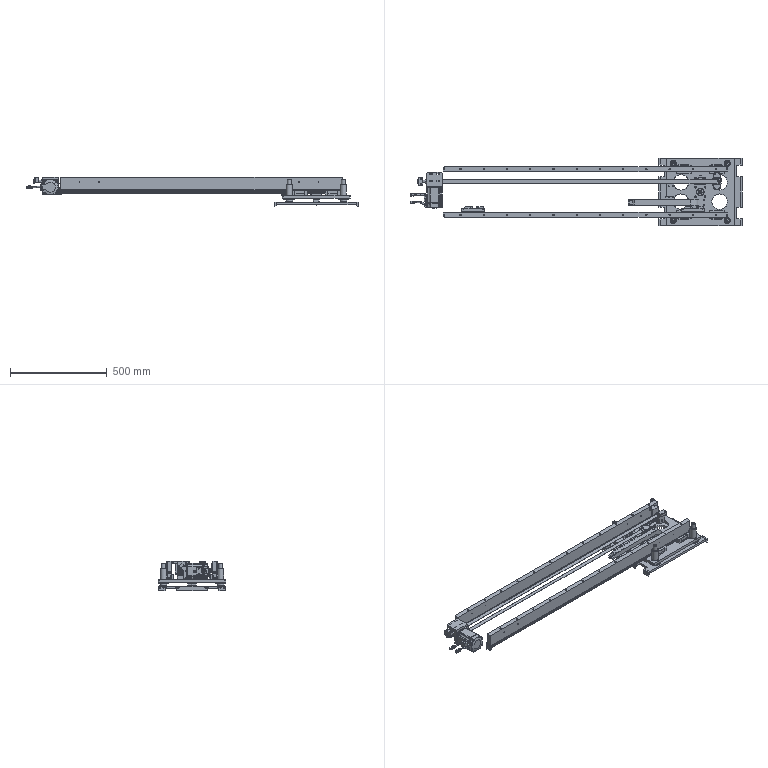Part | NX | 77 solids | 4581 faces | volume 10269997 mm3 | plane 2725 | cylinder 1381 | spline 306 | cone 169 | commonest cylinder face diameters 1 x126 10 x110 0.8 x109 1.2 x108 4.2 x84 6 x77